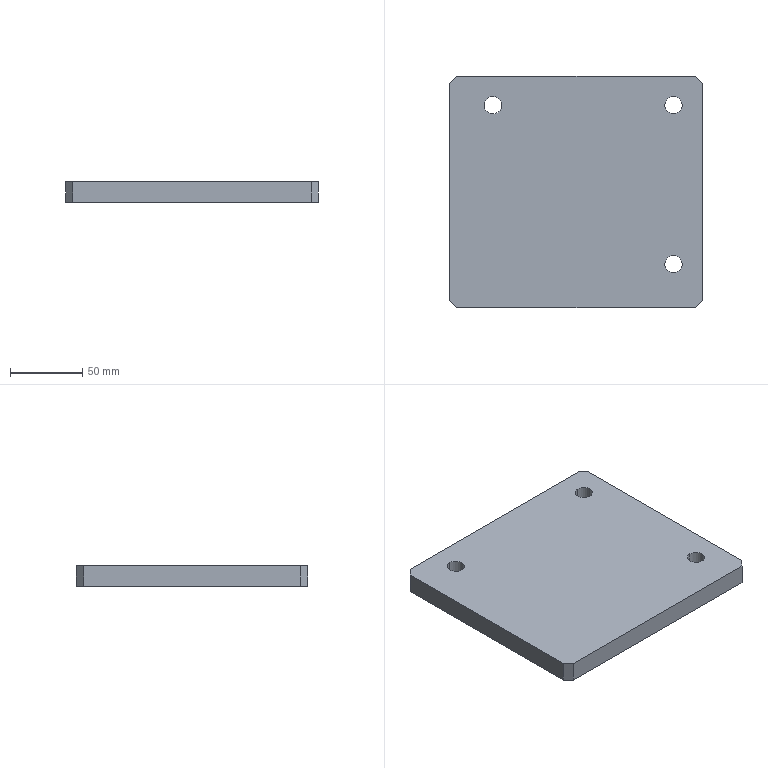Part | STEP file | [08] | 1 solid | 16 faces | box 175 x 160 x 14 mm | volume 386550 mm3 | plane 10 | cylinder 6 | commonest cylinder face diameters 12 x6
STEP:
#1=CARTESIAN_POINT('',(0.,0.,0.));
#2=DIRECTION('',(0.,0.,1.));
#3=DIRECTION('',(1.,0.,0.));
#4=AXIS2_PLACEMENT_3D('',#1,#2,#3);
#5=CARTESIAN_POINT('',(30.,134.,0.));
#6=VERTEX_POINT('',#5);
#7=CARTESIAN_POINT('',(30.,134.,14.));
#8=VERTEX_POINT('',#7);
#9=CARTESIAN_POINT('',(30.,134.,0.));
#10=DIRECTION('',(0.,0.,1.));
#11=VECTOR('',#10,1.);
#12=LINE('',#9,#11);
#13=CARTESIAN_POINT('',(30.,140.,0.));
#14=DIRECTION('',(0.,0.,1.));
#15=DIRECTION('',(0.,-1.,0.));
#16=AXIS2_PLACEMENT_3D('',#13,#14,#15);
#17=CYLINDRICAL_SURFACE('',#16,6.);
#18=CARTESIAN_POINT('',(6.283,0.));
#19=DIRECTION('',(0.,1.));
#20=VECTOR('',#19,1.);
#21=LINE('',#18,#20);
#22=(GEOMETRIC_REPRESENTATION_CONTEXT(2)PARAMETRIC_REPRESENTATION_CONTEXT()REPRESENTATION_CONTEXT('',''));
#23=DEFINITIONAL_REPRESENTATION('',(#21),#22);
#24=PCURVE('',#17,#23);
#25=CARTESIAN_POINT('',(30.,140.,0.));
#26=DIRECTION('',(0.,0.,1.));
#27=DIRECTION('',(0.,-1.,0.));
#28=AXIS2_PLACEMENT_3D('',#25,#26,#27);
#29=CYLINDRICAL_SURFACE('',#28,6.);
#30=CARTESIAN_POINT('',(0.,0.));
#31=DIRECTION('',(0.,1.));
#32=VECTOR('',#31,1.);
#33=LINE('',#30,#32);
#34=(GEOMETRIC_REPRESENTATION_CONTEXT(2)PARAMETRIC_REPRESENTATION_CONTEXT()REPRESENTATION_CONTEXT('',''));
#35=DEFINITIONAL_REPRESENTATION('',(#33),#34);
#36=PCURVE('',#29,#35);
#37=SURFACE_CURVE('',#12,(#24,#36),.PCURVE_S1.);
#38=EDGE_CURVE('',#6,#8,#37,.T.);
#39=ORIENTED_EDGE('',*,*,#38,.T.);
#40=CARTESIAN_POINT('',(30.,146.,14.));
#41=VERTEX_POINT('',#40);
#42=CARTESIAN_POINT('',(30.,140.,14.));
#43=DIRECTION('',(0.,0.,-1.));
#44=DIRECTION('',(0.,1.,0.));
#45=AXIS2_PLACEMENT_3D('',#42,#43,#44);
#46=CIRCLE('',#45,6.);
#47=CARTESIAN_POINT('',(9.425,14.));
#48=DIRECTION('',(-1.,0.));
#49=VECTOR('',#48,1.);
#50=LINE('',#47,#49);
#51=(GEOMETRIC_REPRESENTATION_CONTEXT(2)PARAMETRIC_REPRESENTATION_CONTEXT()REPRESENTATION_CONTEXT('',''));
#52=DEFINITIONAL_REPRESENTATION('',(#50),#51);
#53=PCURVE('',#17,#52);
#54=CARTESIAN_POINT('',(87.5,80.,14.));
#55=DIRECTION('',(0.,0.,1.));
#56=DIRECTION('',(0.,-1.,0.));
#57=AXIS2_PLACEMENT_3D('',#54,#55,#56);
#58=PLANE('',#57);
#59=CARTESIAN_POINT('',(-66.,-57.5));
#60=CARTESIAN_POINT('',(-66.,-47.108));
#61=CARTESIAN_POINT('',(-57.,-52.304));
#62=CARTESIAN_POINT('',(-48.,-57.5));
#63=CARTESIAN_POINT('',(-57.,-62.696));
#64=CARTESIAN_POINT('',(-66.,-67.892));
#65=CARTESIAN_POINT('',(-66.,-57.5));
#66=(BOUNDED_CURVE()B_SPLINE_CURVE(2,(#59,#60,#61,#62,#63,#64,#65),.UNSPECIFIED.,.T.,.F.)B_SPLINE_CURVE_WITH_KNOTS((1,2,2,2,2,1),(-2.094,0.,2.094,4.189,6.283,8.378),.UNSPECIFIED.)CURVE()GEOMETRIC_REPRESENTATION_ITEM()RATIONAL_B_SPLINE_CURVE((1.,0.5,1.,0.5,1.,0.5,1.))REPRESENTATION_ITEM(''));
#67=(GEOMETRIC_REPRESENTATION_CONTEXT(2)PARAMETRIC_REPRESENTATION_CONTEXT()REPRESENTATION_CONTEXT('',''));
#68=DEFINITIONAL_REPRESENTATION('',(#66),#67);
#69=PCURVE('',#58,#68);
#70=SURFACE_CURVE('',#46,(#53,#69),.PCURVE_S1.);
#71=EDGE_CURVE('',#8,#41,#70,.T.);
#72=ORIENTED_EDGE('',*,*,#71,.T.);
#73=CARTESIAN_POINT('',(30.,146.,0.));
#74=VERTEX_POINT('',#73);
#75=CARTESIAN_POINT('',(30.,146.,0.));
#76=DIRECTION('',(0.,0.,1.));
#77=VECTOR('',#76,1.);
#78=LINE('',#75,#77);
#79=CARTESIAN_POINT('',(3.142,0.));
#80=DIRECTION('',(0.,1.));
#81=VECTOR('',#80,1.);
#82=LINE('',#79,#81);
#83=(GEOMETRIC_REPRESENTATION_CONTEXT(2)PARAMETRIC_REPRESENTATION_CONTEXT()REPRESENTATION_CONTEXT('',''));
#84=DEFINITIONAL_REPRESENTATION('',(#82),#83);
#85=PCURVE('',#17,#84);
#86=CARTESIAN_POINT('',(3.142,0.));
#87=DIRECTION('',(0.,1.));
#88=VECTOR('',#87,1.);
#89=LINE('',#86,#88);
#90=(GEOMETRIC_REPRESENTATION_CONTEXT(2)PARAMETRIC_REPRESENTATION_CONTEXT()REPRESENTATION_CONTEXT('',''));
#91=DEFINITIONAL_REPRESENTATION('',(#89),#90);
#92=PCURVE('',#29,#91);
#93=SURFACE_CURVE('',#78,(#85,#92),.PCURVE_S1.);
#94=EDGE_CURVE('',#74,#41,#93,.T.);
#95=ORIENTED_EDGE('',*,*,#94,.F.);
#96=CARTESIAN_POINT('',(30.,140.,0.));
#97=DIRECTION('',(0.,0.,1.));
#98=DIRECTION('',(0.,-1.,0.));
#99=AXIS2_PLACEMENT_3D('',#96,#97,#98);
#100=CIRCLE('',#99,6.);
#101=CARTESIAN_POINT('',(0.,0.));
#102=DIRECTION('',(1.,0.));
#103=VECTOR('',#102,1.);
#104=LINE('',#101,#103);
#105=(GEOMETRIC_REPRESENTATION_CONTEXT(2)PARAMETRIC_REPRESENTATION_CONTEXT()REPRESENTATION_CONTEXT('',''));
#106=DEFINITIONAL_REPRESENTATION('',(#104),#105);
#107=PCURVE('',#17,#106);
#108=CARTESIAN_POINT('',(87.5,80.,0.));
#109=DIRECTION('',(0.,0.,-1.));
#110=DIRECTION('',(0.,1.,0.));
#111=AXIS2_PLACEMENT_3D('',#108,#109,#110);
#112=PLANE('',#111);
#113=CARTESIAN_POINT('',(54.,-57.5));
#114=CARTESIAN_POINT('',(54.,-47.108));
#115=CARTESIAN_POINT('',(63.,-52.304));
#116=CARTESIAN_POINT('',(72.,-57.5));
#117=CARTESIAN_POINT('',(63.,-62.696));
#118=CARTESIAN_POINT('',(54.,-67.892));
#119=CARTESIAN_POINT('',(54.,-57.5));
#120=(BOUNDED_CURVE()B_SPLINE_CURVE(2,(#113,#114,#115,#116,#117,#118,#119),.UNSPECIFIED.,.T.,.F.)B_SPLINE_CURVE_WITH_KNOTS((1,2,2,2,2,1),(-2.094,0.,2.094,4.189,6.283,8.378),.UNSPECIFIED.)CURVE()GEOMETRIC_REPRESENTATION_ITEM()RATIONAL_B_SPLINE_CURVE((1.,0.5,1.,0.5,1.,0.5,1.))REPRESENTATION_ITEM(''));
#121=(GEOMETRIC_REPRESENTATION_CONTEXT(2)PARAMETRIC_REPRESENTATION_CONTEXT()REPRESENTATION_CONTEXT('',''));
#122=DEFINITIONAL_REPRESENTATION('',(#120),#121);
#123=PCURVE('',#112,#122);
#124=SURFACE_CURVE('',#100,(#107,#123),.PCURVE_S1.);
#125=EDGE_CURVE('',#74,#6,#124,.T.);
#126=ORIENTED_EDGE('',*,*,#125,.T.);
#127=EDGE_LOOP('',(#39,#72,#95,#126));
#128=FACE_BOUND('',#127,.F.);
#129=ADVANCED_FACE('',(#128),#17,.F.);
#130=CARTESIAN_POINT('',(155.,24.,0.));
#131=VERTEX_POINT('',#130);
#132=CARTESIAN_POINT('',(155.,24.,14.));
#133=VERTEX_POINT('',#132);
#134=CARTESIAN_POINT('',(155.,24.,0.));
#135=DIRECTION('',(0.,0.,1.));
#136=VECTOR('',#135,1.);
#137=LINE('',#134,#136);
#138=CARTESIAN_POINT('',(155.,30.,0.));
#139=DIRECTION('',(0.,0.,1.));
#140=DIRECTION('',(0.,-1.,0.));
#141=AXIS2_PLACEMENT_3D('',#138,#139,#140);
#142=CYLINDRICAL_SURFACE('',#141,6.);
#143=CARTESIAN_POINT('',(6.283,0.));
#144=DIRECTION('',(0.,1.));
#145=VECTOR('',#144,1.);
#146=LINE('',#143,#145);
#147=(GEOMETRIC_REPRESENTATION_CONTEXT(2)PARAMETRIC_REPRESENTATION_CONTEXT()REPRESENTATION_CONTEXT('',''));
#148=DEFINITIONAL_REPRESENTATION('',(#146),#147);
#149=PCURVE('',#142,#148);
#150=CARTESIAN_POINT('',(155.,30.,0.));
#151=DIRECTION('',(0.,0.,1.));
#152=DIRECTION('',(0.,-1.,0.));
#153=AXIS2_PLACEMENT_3D('',#150,#151,#152);
#154=CYLINDRICAL_SURFACE('',#153,6.);
#155=CARTESIAN_POINT('',(0.,0.));
#156=DIRECTION('',(0.,1.));
#157=VECTOR('',#156,1.);
#158=LINE('',#155,#157);
#159=(GEOMETRIC_REPRESENTATION_CONTEXT(2)PARAMETRIC_REPRESENTATION_CONTEXT()REPRESENTATION_CONTEXT('',''));
#160=DEFINITIONAL_REPRESENTATION('',(#158),#159);
#161=PCURVE('',#154,#160);
#162=SURFACE_CURVE('',#137,(#149,#161),.PCURVE_S1.);
#163=EDGE_CURVE('',#131,#133,#162,.T.);
#164=ORIENTED_EDGE('',*,*,#163,.T.);
#165=CARTESIAN_POINT('',(155.,36.,14.));
#166=VERTEX_POINT('',#165);
#167=CARTESIAN_POINT('',(155.,30.,14.));
#168=DIRECTION('',(0.,0.,-1.));
#169=DIRECTION('',(0.,1.,0.));
#170=AXIS2_PLACEMENT_3D('',#167,#168,#169);
#171=CIRCLE('',#170,6.);
#172=CARTESIAN_POINT('',(9.425,14.));
#173=DIRECTION('',(-1.,0.));
#174=VECTOR('',#173,1.);
#175=LINE('',#172,#174);
#176=(GEOMETRIC_REPRESENTATION_CONTEXT(2)PARAMETRIC_REPRESENTATION_CONTEXT()REPRESENTATION_CONTEXT('',''));
#177=DEFINITIONAL_REPRESENTATION('',(#175),#176);
#178=PCURVE('',#142,#177);
#179=CARTESIAN_POINT('',(44.,67.5));
#180=CARTESIAN_POINT('',(44.,77.892));
#181=CARTESIAN_POINT('',(53.,72.696));
#182=CARTESIAN_POINT('',(62.,67.5));
#183=CARTESIAN_POINT('',(53.,62.304));
#184=CARTESIAN_POINT('',(44.,57.108));
#185=CARTESIAN_POINT('',(44.,67.5));
#186=(BOUNDED_CURVE()B_SPLINE_CURVE(2,(#179,#180,#181,#182,#183,#184,#185),.UNSPECIFIED.,.T.,.F.)B_SPLINE_CURVE_WITH_KNOTS((1,2,2,2,2,1),(-2.094,0.,2.094,4.189,6.283,8.378),.UNSPECIFIED.)CURVE()GEOMETRIC_REPRESENTATION_ITEM()RATIONAL_B_SPLINE_CURVE((1.,0.5,1.,0.5,1.,0.5,1.))REPRESENTATION_ITEM(''));
#187=(GEOMETRIC_REPRESENTATION_CONTEXT(2)PARAMETRIC_REPRESENTATION_CONTEXT()REPRESENTATION_CONTEXT('',''));
#188=DEFINITIONAL_REPRESENTATION('',(#186),#187);
#189=PCURVE('',#58,#188);
#190=SURFACE_CURVE('',#171,(#178,#189),.PCURVE_S1.);
#191=EDGE_CURVE('',#133,#166,#190,.T.);
#192=ORIENTED_EDGE('',*,*,#191,.T.);
#193=CARTESIAN_POINT('',(155.,36.,0.));
#194=VERTEX_POINT('',#193);
#195=CARTESIAN_POINT('',(155.,36.,0.));
#196=DIRECTION('',(0.,0.,1.));
#197=VECTOR('',#196,1.);
#198=LINE('',#195,#197);
#199=CARTESIAN_POINT('',(3.142,0.));
#200=DIRECTION('',(0.,1.));
#201=VECTOR('',#200,1.);
#202=LINE('',#199,#201);
#203=(GEOMETRIC_REPRESENTATION_CONTEXT(2)PARAMETRIC_REPRESENTATION_CONTEXT()REPRESENTATION_CONTEXT('',''));
#204=DEFINITIONAL_REPRESENTATION('',(#202),#203);
#205=PCURVE('',#142,#204);
#206=CARTESIAN_POINT('',(3.142,0.));
#207=DIRECTION('',(0.,1.));
#208=VECTOR('',#207,1.);
#209=LINE('',#206,#208);
#210=(GEOMETRIC_REPRESENTATION_CONTEXT(2)PARAMETRIC_REPRESENTATION_CONTEXT()REPRESENTATION_CONTEXT('',''));
#211=DEFINITIONAL_REPRESENTATION('',(#209),#210);
#212=PCURVE('',#154,#211);
#213=SURFACE_CURVE('',#198,(#205,#212),.PCURVE_S1.);
#214=EDGE_CURVE('',#194,#166,#213,.T.);
#215=ORIENTED_EDGE('',*,*,#214,.F.);
#216=CARTESIAN_POINT('',(155.,30.,0.));
#217=DIRECTION('',(0.,0.,1.));
#218=DIRECTION('',(0.,-1.,0.));
#219=AXIS2_PLACEMENT_3D('',#216,#217,#218);
#220=CIRCLE('',#219,6.);
#221=CARTESIAN_POINT('',(0.,0.));
#222=DIRECTION('',(1.,0.));
#223=VECTOR('',#222,1.);
#224=LINE('',#221,#223);
#225=(GEOMETRIC_REPRESENTATION_CONTEXT(2)PARAMETRIC_REPRESENTATION_CONTEXT()REPRESENTATION_CONTEXT('',''));
#226=DEFINITIONAL_REPRESENTATION('',(#224),#225);
#227=PCURVE('',#142,#226);
#228=CARTESIAN_POINT('',(-56.,67.5));
#229=CARTESIAN_POINT('',(-56.,77.892));
#230=CARTESIAN_POINT('',(-47.,72.696));
#231=CARTESIAN_POINT('',(-38.,67.5));
#232=CARTESIAN_POINT('',(-47.,62.304));
#233=CARTESIAN_POINT('',(-56.,57.108));
#234=CARTESIAN_POINT('',(-56.,67.5));
#235=(BOUNDED_CURVE()B_SPLINE_CURVE(2,(#228,#229,#230,#231,#232,#233,#234),.UNSPECIFIED.,.T.,.F.)B_SPLINE_CURVE_WITH_KNOTS((1,2,2,2,2,1),(-2.094,0.,2.094,4.189,6.283,8.378),.UNSPECIFIED.)CURVE()GEOMETRIC_REPRESENTATION_ITEM()RATIONAL_B_SPLINE_CURVE((1.,0.5,1.,0.5,1.,0.5,1.))REPRESENTATION_ITEM(''));
#236=(GEOMETRIC_REPRESENTATION_CONTEXT(2)PARAMETRIC_REPRESENTATION_CONTEXT()REPRESENTATION_CONTEXT('',''));
#237=DEFINITIONAL_REPRESENTATION('',(#235),#236);
#238=PCURVE('',#112,#237);
#239=SURFACE_CURVE('',#220,(#227,#238),.PCURVE_S1.);
#240=EDGE_CURVE('',#194,#131,#239,.T.);
#241=ORIENTED_EDGE('',*,*,#240,.T.);
#242=EDGE_LOOP('',(#164,#192,#215,#241));
#243=FACE_BOUND('',#242,.F.);
#244=ADVANCED_FACE('',(#243),#142,.F.);
#245=CARTESIAN_POINT('',(155.,134.,0.));
#246=VERTEX_POINT('',#245);
#247=CARTESIAN_POINT('',(155.,134.,14.));
#248=VERTEX_POINT('',#247);
#249=CARTESIAN_POINT('',(155.,134.,0.));
#250=DIRECTION('',(0.,0.,1.));
#251=VECTOR('',#250,1.);
#252=LINE('',#249,#251);
#253=CARTESIAN_POINT('',(155.,140.,0.));
#254=DIRECTION('',(0.,0.,1.));
#255=DIRECTION('',(0.,-1.,0.));
#256=AXIS2_PLACEMENT_3D('',#253,#254,#255);
#257=CYLINDRICAL_SURFACE('',#256,6.);
#258=CARTESIAN_POINT('',(6.283,0.));
#259=DIRECTION('',(0.,1.));
#260=VECTOR('',#259,1.);
#261=LINE('',#258,#260);
#262=(GEOMETRIC_REPRESENTATION_CONTEXT(2)PARAMETRIC_REPRESENTATION_CONTEXT()REPRESENTATION_CONTEXT('',''));
#263=DEFINITIONAL_REPRESENTATION('',(#261),#262);
#264=PCURVE('',#257,#263);
#265=CARTESIAN_POINT('',(155.,140.,0.));
#266=DIRECTION('',(0.,0.,1.));
#267=DIRECTION('',(0.,-1.,0.));
#268=AXIS2_PLACEMENT_3D('',#265,#266,#267);
#269=CYLINDRICAL_SURFACE('',#268,6.);
#270=CARTESIAN_POINT('',(0.,0.));
#271=DIRECTION('',(0.,1.));
#272=VECTOR('',#271,1.);
#273=LINE('',#270,#272);
#274=(GEOMETRIC_REPRESENTATION_CONTEXT(2)PARAMETRIC_REPRESENTATION_CONTEXT()REPRESENTATION_CONTEXT('',''));
#275=DEFINITIONAL_REPRESENTATION('',(#273),#274);
#276=PCURVE('',#269,#275);
#277=SURFACE_CURVE('',#252,(#264,#276),.PCURVE_S1.);
#278=EDGE_CURVE('',#246,#248,#277,.T.);
#279=ORIENTED_EDGE('',*,*,#278,.T.);
#280=CARTESIAN_POINT('',(155.,146.,14.));
#281=VERTEX_POINT('',#280);
#282=CARTESIAN_POINT('',(155.,140.,14.));
#283=DIRECTION('',(0.,0.,-1.));
#284=DIRECTION('',(0.,1.,0.));
#285=AXIS2_PLACEMENT_3D('',#282,#283,#284);
#286=CIRCLE('',#285,6.);
#287=CARTESIAN_POINT('',(9.425,14.));
#288=DIRECTION('',(-1.,0.));
#289=VECTOR('',#288,1.);
#290=LINE('',#287,#289);
#291=(GEOMETRIC_REPRESENTATION_CONTEXT(2)PARAMETRIC_REPRESENTATION_CONTEXT()REPRESENTATION_CONTEXT('',''));
#292=DEFINITIONAL_REPRESENTATION('',(#290),#291);
#293=PCURVE('',#257,#292);
#294=CARTESIAN_POINT('',(-66.,67.5));
#295=CARTESIAN_POINT('',(-66.,77.892));
#296=CARTESIAN_POINT('',(-57.,72.696));
#297=CARTESIAN_POINT('',(-48.,67.5));
#298=CARTESIAN_POINT('',(-57.,62.304));
#299=CARTESIAN_POINT('',(-66.,57.108));
#300=CARTESIAN_POINT('',(-66.,67.5));
#301=(BOUNDED_CURVE()B_SPLINE_CURVE(2,(#294,#295,#296,#297,#298,#299,#300),.UNSPECIFIED.,.T.,.F.)B_SPLINE_CURVE_WITH_KNOTS((1,2,2,2,2,1),(-2.094,0.,2.094,4.189,6.283,8.378),.UNSPECIFIED.)CURVE()GEOMETRIC_REPRESENTATION_ITEM()RATIONAL_B_SPLINE_CURVE((1.,0.5,1.,0.5,1.,0.5,1.))REPRESENTATION_ITEM(''));
#302=(GEOMETRIC_REPRESENTATION_CONTEXT(2)PARAMETRIC_REPRESENTATION_CONTEXT()REPRESENTATION_CONTEXT('',''));
#303=DEFINITIONAL_REPRESENTATION('',(#301),#302);
#304=PCURVE('',#58,#303);
#305=SURFACE_CURVE('',#286,(#293,#304),.PCURVE_S1.);
#306=EDGE_CURVE('',#248,#281,#305,.T.);
#307=ORIENTED_EDGE('',*,*,#306,.T.);
#308=CARTESIAN_POINT('',(155.,146.,0.));
#309=VERTEX_POINT('',#308);
#310=CARTESIAN_POINT('',(155.,146.,0.));
#311=DIRECTION('',(0.,0.,1.));
#312=VECTOR('',#311,1.);
#313=LINE('',#310,#312);
#314=CARTESIAN_POINT('',(3.142,0.));
#315=DIRECTION('',(0.,1.));
#316=VECTOR('',#315,1.);
#317=LINE('',#314,#316);
#318=(GEOMETRIC_REPRESENTATION_CONTEXT(2)PARAMETRIC_REPRESENTATION_CONTEXT()REPRESENTATION_CONTEXT('',''));
#319=DEFINITIONAL_REPRESENTATION('',(#317),#318);
#320=PCURVE('',#257,#319);
#321=CARTESIAN_POINT('',(3.142,0.));
#322=DIRECTION('',(0.,1.));
#323=VECTOR('',#322,1.);
#324=LINE('',#321,#323);
#325=(GEOMETRIC_REPRESENTATION_CONTEXT(2)PARAMETRIC_REPRESENTATION_CONTEXT()REPRESENTATION_CONTEXT('',''));
#326=DEFINITIONAL_REPRESENTATION('',(#324),#325);
#327=PCURVE('',#269,#326);
#328=SURFACE_CURVE('',#313,(#320,#327),.PCURVE_S1.);
#329=EDGE_CURVE('',#309,#281,#328,.T.);
#330=ORIENTED_EDGE('',*,*,#329,.F.);
#331=CARTESIAN_POINT('',(155.,140.,0.));
#332=DIRECTION('',(0.,0.,1.));
#333=DIRECTION('',(0.,-1.,0.));
#334=AXIS2_PLACEMENT_3D('',#331,#332,#333);
#335=CIRCLE('',#334,6.);
#336=CARTESIAN_POINT('',(0.,0.));
#337=DIRECTION('',(1.,0.));
#338=VECTOR('',#337,1.);
#339=LINE('',#336,#338);
#340=(GEOMETRIC_REPRESENTATION_CONTEXT(2)PARAMETRIC_REPRESENTATION_CONTEXT()REPRESENTATION_CONTEXT('',''));
#341=DEFINITIONAL_REPRESENTATION('',(#339),#340);
#342=PCURVE('',#257,#341);
#343=CARTESIAN_POINT('',(54.,67.5));
#344=CARTESIAN_POINT('',(54.,77.892));
#345=CARTESIAN_POINT('',(63.,72.696));
#346=CARTESIAN_POINT('',(72.,67.5));
#347=CARTESIAN_POINT('',(63.,62.304));
#348=CARTESIAN_POINT('',(54.,57.108));
#349=CARTESIAN_POINT('',(54.,67.5));
#350=(BOUNDED_CURVE()B_SPLINE_CURVE(2,(#343,#344,#345,#346,#347,#348,#349),.UNSPECIFIED.,.T.,.F.)B_SPLINE_CURVE_WITH_KNOTS((1,2,2,2,2,1),(-2.094,0.,2.094,4.189,6.283,8.378),.UNSPECIFIED.)CURVE()GEOMETRIC_REPRESENTATION_ITEM()RATIONAL_B_SPLINE_CURVE((1.,0.5,1.,0.5,1.,0.5,1.))REPRESENTATION_ITEM(''));
#351=(GEOMETRIC_REPRESENTATION_CONTEXT(2)PARAMETRIC_REPRESENTATION_CONTEXT()REPRESENTATION_CONTEXT('',''));
#352=DEFINITIONAL_REPRESENTATION('',(#350),#351);
#353=PCURVE('',#112,#352);
#354=SURFACE_CURVE('',#335,(#342,#353),.PCURVE_S1.);
#355=EDGE_CURVE('',#309,#246,#354,.T.);
#356=ORIENTED_EDGE('',*,*,#355,.T.);
#357=EDGE_LOOP('',(#279,#307,#330,#356));
#358=FACE_BOUND('',#357,.F.);
#359=ADVANCED_FACE('',(#358),#257,.F.);
#360=ORIENTED_EDGE('',*,*,#71,.T.);
#361=CARTESIAN_POINT('',(30.,140.,14.));
#362=DIRECTION('',(0.,0.,-1.));
#363=DIRECTION('',(0.,1.,0.));
#364=AXIS2_PLACEMENT_3D('',#361,#362,#363);
#365=CIRCLE('',#364,6.);
#366=CARTESIAN_POINT('',(-66.,-57.5));
#367=CARTESIAN_POINT('',(-66.,-47.108));
#368=CARTESIAN_POINT('',(-57.,-52.304));
#369=CARTESIAN_POINT('',(-48.,-57.5));
#370=CARTESIAN_POINT('',(-57.,-62.696));
#371=CARTESIAN_POINT('',(-66.,-67.892));
#372=CARTESIAN_POINT('',(-66.,-57.5));
#373=(BOUNDED_CURVE()B_SPLINE_CURVE(2,(#366,#367,#368,#369,#370,#371,#372),.UNSPECIFIED.,.T.,.F.)B_SPLINE_CURVE_WITH_KNOTS((1,2,2,2,2,1),(-2.094,0.,2.094,4.189,6.283,8.378),.UNSPECIFIED.)CURVE()GEOMETRIC_REPRESENTATION_ITEM()RATIONAL_B_SPLINE_CURVE((1.,0.5,1.,0.5,1.,0.5,1.))REPRESENTATION_ITEM(''));
#374=(GEOMETRIC_REPRESENTATION_CONTEXT(2)PARAMETRIC_REPRESENTATION_CONTEXT()REPRESENTATION_CONTEXT('',''));
#375=DEFINITIONAL_REPRESENTATION('',(#373),#374);
#376=PCURVE('',#58,#375);
#377=CARTESIAN_POINT('',(3.142,14.));
#378=DIRECTION('',(-1.,0.));
#379=VECTOR('',#378,1.);
#380=LINE('',#377,#379);
#381=(GEOMETRIC_REPRESENTATION_CONTEXT(2)PARAMETRIC_REPRESENTATION_CONTEXT()REPRESENTATION_CONTEXT('',''));
#382=DEFINITIONAL_REPRESENTATION('',(#380),#381);
#383=PCURVE('',#29,#382);
#384=SURFACE_CURVE('',#365,(#376,#383),.PCURVE_S1.);
#385=EDGE_CURVE('',#41,#8,#384,.T.);
#386=ORIENTED_EDGE('',*,*,#385,.T.);
#387=EDGE_LOOP('',(#360,#386));
#388=FACE_BOUND('',#387,.T.);
#389=ORIENTED_EDGE('',*,*,#191,.T.);
#390=CARTESIAN_POINT('',(155.,30.,14.));
#391=DIRECTION('',(0.,0.,-1.));
#392=DIRECTION('',(0.,1.,0.));
#393=AXIS2_PLACEMENT_3D('',#390,#391,#392);
#394=CIRCLE('',#393,6.);
#395=CARTESIAN_POINT('',(44.,67.5));
#396=CARTESIAN_POINT('',(44.,77.892));
#397=CARTESIAN_POINT('',(53.,72.696));
#398=CARTESIAN_POINT('',(62.,67.5));
#399=CARTESIAN_POINT('',(53.,62.304));
#400=CARTESIAN_POINT('',(44.,57.108));
#401=CARTESIAN_POINT('',(44.,67.5));
#402=(BOUNDED_CURVE()B_SPLINE_CURVE(2,(#395,#396,#397,#398,#399,#400,#401),.UNSPECIFIED.,.T.,.F.)B_SPLINE_CURVE_WITH_KNOTS((1,2,2,2,2,1),(-2.094,0.,2.094,4.189,6.283,8.378),.UNSPECIFIED.)CURVE()GEOMETRIC_REPRESENTATION_ITEM()RATIONAL_B_SPLINE_CURVE((1.,0.5,1.,0.5,1.,0.5,1.))REPRESENTATION_ITEM(''));
#403=(GEOMETRIC_REPRESENTATION_CONTEXT(2)PARAMETRIC_REPRESENTATION_CONTEXT()REPRESENTATION_CONTEXT('',''));
#404=DEFINITIONAL_REPRESENTATION('',(#402),#403);
#405=PCURVE('',#58,#404);
#406=CARTESIAN_POINT('',(3.142,14.));
#407=DIRECTION('',(-1.,0.));
#408=VECTOR('',#407,1.);
#409=LINE('',#406,#408);
#410=(GEOMETRIC_REPRESENTATION_CONTEXT(2)PARAMETRIC_REPRESENTATION_CONTEXT()REPRESENTATION_CONTEXT('',''));
#411=DEFINITIONAL_REPRESENTATION('',(#409),#410);
#412=PCURVE('',#154,#411);
#413=SURFACE_CURVE('',#394,(#405,#412),.PCURVE_S1.);
#414=EDGE_CURVE('',#166,#133,#413,.T.);
#415=ORIENTED_EDGE('',*,*,#414,.T.);
#416=EDGE_LOOP('',(#389,#415));
#417=FACE_BOUND('',#416,.T.);
#418=ORIENTED_EDGE('',*,*,#306,.T.);
#419=CARTESIAN_POINT('',(155.,140.,14.));
#420=DIRECTION('',(0.,0.,-1.));
#421=DIRECTION('',(0.,1.,0.));
#422=AXIS2_PLACEMENT_3D('',#419,#420,#421);
#423=CIRCLE('',#422,6.);
#424=CARTESIAN_POINT('',(-66.,67.5));
#425=CARTESIAN_POINT('',(-66.,77.892));
#426=CARTESIAN_POINT('',(-57.,72.696));
#427=CARTESIAN_POINT('',(-48.,67.5));
#428=CARTESIAN_POINT('',(-57.,62.304));
#429=CARTESIAN_POINT('',(-66.,57.108));
#430=CARTESIAN_POINT('',(-66.,67.5));
#431=(BOUNDED_CURVE()B_SPLINE_CURVE(2,(#424,#425,#426,#427,#428,#429,#430),.UNSPECIFIED.,.T.,.F.)B_SPLINE_CURVE_WITH_KNOTS((1,2,2,2,2,1),(-2.094,0.,2.094,4.189,6.283,8.378),.UNSPECIFIED.)CURVE()GEOMETRIC_REPRESENTATION_ITEM()RATIONAL_B_SPLINE_CURVE((1.,0.5,1.,0.5,1.,0.5,1.))REPRESENTATION_ITEM(''));
#432=(GEOMETRIC_REPRESENTATION_CONTEXT(2)PARAMETRIC_REPRESENTATION_CONTEXT()REPRESENTATION_CONTEXT('',''));
#433=DEFINITIONAL_REPRESENTATION('',(#431),#432);
#434=PCURVE('',#58,#433);
#435=CARTESIAN_POINT('',(3.142,14.));
#436=DIRECTION('',(-1.,0.));
#437=VECTOR('',#436,1.);
#438=LINE('',#435,#437);
#439=(GEOMETRIC_REPRESENTATION_CONTEXT(2)PARAMETRIC_REPRESENTATION_CONTEXT()REPRESENTATION_CONTEXT('',''));
#440=DEFINITIONAL_REPRESENTATION('',(#438),#439);
#441=PCURVE('',#269,#440);
#442=SURFACE_CURVE('',#423,(#434,#441),.PCURVE_S1.);
#443=EDGE_CURVE('',#281,#248,#442,.T.);
#444=ORIENTED_EDGE('',*,*,#443,.T.);
#445=EDGE_LOOP('',(#418,#444));
#446=FACE_BOUND('',#445,.T.);
#447=CARTESIAN_POINT('',(170.,0.,14.));
#448=VERTEX_POINT('',#447);
#449=CARTESIAN_POINT('',(5.,0.,14.));
#450=VERTEX_POINT('',#449);
#451=CARTESIAN_POINT('',(87.5,0.,14.));
#452=DIRECTION('',(-1.,0.,0.));
#453=VECTOR('',#452,1.);
#454=LINE('',#451,#453);
#455=CARTESIAN_POINT('',(80.,0.));
#456=DIRECTION('',(0.,-1.));
#457=VECTOR('',#456,1.);
#458=LINE('',#455,#457);
#459=(GEOMETRIC_REPRESENTATION_CONTEXT(2)PARAMETRIC_REPRESENTATION_CONTEXT()REPRESENTATION_CONTEXT('',''));
#460=DEFINITIONAL_REPRESENTATION('',(#458),#459);
#461=PCURVE('',#58,#460);
#462=CARTESIAN_POINT('',(87.5,0.,0.));
#463=DIRECTION('',(0.,-1.,0.));
#464=DIRECTION('',(0.,0.,-1.));
#465=AXIS2_PLACEMENT_3D('',#462,#463,#464);
#466=PLANE('',#465);
#467=CARTESIAN_POINT('',(-14.,0.));
#468=DIRECTION('',(0.,-1.));
#469=VECTOR('',#468,1.);
#470=LINE('',#467,#469);
#471=(GEOMETRIC_REPRESENTATION_CONTEXT(2)PARAMETRIC_REPRESENTATION_CONTEXT()REPRESENTATION_CONTEXT('',''));
#472=DEFINITIONAL_REPRESENTATION('',(#470),#471);
#473=PCURVE('',#466,#472);
#474=SURFACE_CURVE('',#454,(#461,#473),.PCURVE_S1.);
#475=EDGE_CURVE('',#448,#450,#474,.T.);
#476=ORIENTED_EDGE('',*,*,#475,.F.);
#477=CARTESIAN_POINT('',(175.,5.,14.));
#478=VERTEX_POINT('',#477);
#479=CARTESIAN_POINT('',(168.75,-1.25,14.));
#480=DIRECTION('',(0.7071,0.7071,0.));
#481=VECTOR('',#480,1.);
#482=LINE('',#479,#481);
#483=CARTESIAN_POINT('',(81.25,81.25));
#484=DIRECTION('',(-0.7071,0.7071));
#485=VECTOR('',#484,1.);
#486=LINE('',#483,#485);
#487=(GEOMETRIC_REPRESENTATION_CONTEXT(2)PARAMETRIC_REPRESENTATION_CONTEXT()REPRESENTATION_CONTEXT('',''));
#488=DEFINITIONAL_REPRESENTATION('',(#486),#487);
#489=PCURVE('',#58,#488);
#490=CARTESIAN_POINT('',(170.,0.,0.));
#491=DIRECTION('',(-0.7071,0.7071,0.));
#492=DIRECTION('',(0.,0.,1.));
#493=AXIS2_PLACEMENT_3D('',#490,#491,#492);
#494=PLANE('',#493);
#495=CARTESIAN_POINT('',(14.,-1.768));
#496=DIRECTION('',(0.,1.));
#497=VECTOR('',#496,1.);
#498=LINE('',#495,#497);
#499=(GEOMETRIC_REPRESENTATION_CONTEXT(2)PARAMETRIC_REPRESENTATION_CONTEXT()REPRESENTATION_CONTEXT('',''));
#500=DEFINITIONAL_REPRESENTATION('',(#498),#499);
#501=PCURVE('',#494,#500);
#502=SURFACE_CURVE('',#482,(#489,#501),.PCURVE_S1.);
#503=EDGE_CURVE('',#448,#478,#502,.T.);
#504=ORIENTED_EDGE('',*,*,#503,.T.);
#505=CARTESIAN_POINT('',(175.,155.,14.));
#506=VERTEX_POINT('',#505);
#507=CARTESIAN_POINT('',(175.,80.,14.));
#508=DIRECTION('',(0.,-1.,0.));
#509=VECTOR('',#508,1.);
#510=LINE('',#507,#509);
#511=CARTESIAN_POINT('',(0.,87.5));
#512=DIRECTION('',(1.,0.));
#513=VECTOR('',#512,1.);
#514=LINE('',#511,#513);
#515=(GEOMETRIC_REPRESENTATION_CONTEXT(2)PARAMETRIC_REPRESENTATION_CONTEXT()REPRESENTATION_CONTEXT('',''));
#516=DEFINITIONAL_REPRESENTATION('',(#514),#515);
#517=PCURVE('',#58,#516);
#518=CARTESIAN_POINT('',(175.,80.,0.));
#519=DIRECTION('',(1.,0.,0.));
#520=DIRECTION('',(0.,0.,1.));
#521=AXIS2_PLACEMENT_3D('',#518,#519,#520);
#522=PLANE('',#521);
#523=CARTESIAN_POINT('',(14.,0.));
#524=DIRECTION('',(0.,1.));
#525=VECTOR('',#524,1.);
#526=LINE('',#523,#525);
#527=(GEOMETRIC_REPRESENTATION_CONTEXT(2)PARAMETRIC_REPRESENTATION_CONTEXT()REPRESENTATION_CONTEXT('',''));
#528=DEFINITIONAL_REPRESENTATION('',(#526),#527);
#529=PCURVE('',#522,#528);
#530=SURFACE_CURVE('',#510,(#517,#529),.PCURVE_S1.);
#531=EDGE_CURVE('',#506,#478,#530,.T.);
#532=ORIENTED_EDGE('',*,*,#531,.F.);
#533=CARTESIAN_POINT('',(170.,160.,14.));
#534=VERTEX_POINT('',#533);
#535=CARTESIAN_POINT('',(168.75,161.25,14.));
#536=DIRECTION('',(-0.7071,0.7071,0.));
#537=VECTOR('',#536,1.);
#538=LINE('',#535,#537);
#539=CARTESIAN_POINT('',(-81.25,81.25));
#540=DIRECTION('',(-0.7071,-0.7071));
#541=VECTOR('',#540,1.);
#542=LINE('',#539,#541);
#543=(GEOMETRIC_REPRESENTATION_CONTEXT(2)PARAMETRIC_REPRESENTATION_CONTEXT()REPRESENTATION_CONTEXT('',''));
#544=DEFINITIONAL_REPRESENTATION('',(#542),#543);
#545=PCURVE('',#58,#544);
#546=CARTESIAN_POINT('',(175.,155.,0.));
#547=DIRECTION('',(-0.7071,-0.7071,0.));
#548=DIRECTION('',(0.,0.,1.));
#549=AXIS2_PLACEMENT_3D('',#546,#547,#548);
#550=PLANE('',#549);
#551=CARTESIAN_POINT('',(14.,8.839));
#552=DIRECTION('',(0.,1.));
#553=VECTOR('',#552,1.);
#554=LINE('',#551,#553);
#555=(GEOMETRIC_REPRESENTATION_CONTEXT(2)PARAMETRIC_REPRESENTATION_CONTEXT()REPRESENTATION_CONTEXT('',''));
#556=DEFINITIONAL_REPRESENTATION('',(#554),#555);
#557=PCURVE('',#550,#556);
#558=SURFACE_CURVE('',#538,(#545,#557),.PCURVE_S1.);
#559=EDGE_CURVE('',#506,#534,#558,.T.);
#560=ORIENTED_EDGE('',*,*,#559,.T.);
#561=CARTESIAN_POINT('',(5.,160.,14.));
#562=VERTEX_POINT('',#561);
#563=CARTESIAN_POINT('',(87.5,160.,14.));
#564=DIRECTION('',(1.,0.,0.));
#565=VECTOR('',#564,1.);
#566=LINE('',#563,#565);
#567=CARTESIAN_POINT('',(-80.,0.));
#568=DIRECTION('',(0.,1.));
#569=VECTOR('',#568,1.);
#570=LINE('',#567,#569);
#571=(GEOMETRIC_REPRESENTATION_CONTEXT(2)PARAMETRIC_REPRESENTATION_CONTEXT()REPRESENTATION_CONTEXT('',''));
#572=DEFINITIONAL_REPRESENTATION('',(#570),#571);
#573=PCURVE('',#58,#572);
#574=CARTESIAN_POINT('',(87.5,160.,0.));
#575=DIRECTION('',(0.,1.,0.));
#576=DIRECTION('',(0.,0.,1.));
#577=AXIS2_PLACEMENT_3D('',#574,#575,#576);
#578=PLANE('',#577);
#579=CARTESIAN_POINT('',(14.,0.));
#580=DIRECTION('',(0.,1.));
#581=VECTOR('',#580,1.);
#582=LINE('',#579,#581);
#583=(GEOMETRIC_REPRESENTATION_CONTEXT(2)PARAMETRIC_REPRESENTATION_CONTEXT()REPRESENTATION_CONTEXT('',''));
#584=DEFINITIONAL_REPRESENTATION('',(#582),#583);
#585=PCURVE('',#578,#584);
#586=SURFACE_CURVE('',#566,(#573,#585),.PCURVE_S1.);
#587=EDGE_CURVE('',#562,#534,#586,.T.);
#588=ORIENTED_EDGE('',*,*,#587,.F.);
#589=CARTESIAN_POINT('',(0.,155.,14.));
#590=VERTEX_POINT('',#589);
#591=CARTESIAN_POINT('',(6.25,161.25,14.));
#592=DIRECTION('',(-0.7071,-0.7071,0.));
#593=VECTOR('',#592,1.);
#594=LINE('',#591,#593);
#595=CARTESIAN_POINT('',(-81.25,-81.25));
#596=DIRECTION('',(0.7071,-0.7071));
#597=VECTOR('',#596,1.);
#598=LINE('',#595,#597);
#599=(GEOMETRIC_REPRESENTATION_CONTEXT(2)PARAMETRIC_REPRESENTATION_CONTEXT()REPRESENTATION_CONTEXT('',''));
#600=DEFINITIONAL_REPRESENTATION('',(#598),#599);
#601=PCURVE('',#58,#600);
#602=CARTESIAN_POINT('',(5.,160.,0.));
#603=DIRECTION('',(0.7071,-0.7071,0.));
#604=DIRECTION('',(0.,0.,1.));
#605=AXIS2_PLACEMENT_3D('',#602,#603,#604);
#606=PLANE('',#605);
#607=CARTESIAN_POINT('',(14.,-1.768));
#608=DIRECTION('',(0.,1.));
#609=VECTOR('',#608,1.);
#610=LINE('',#607,#609);
#611=(GEOMETRIC_REPRESENTATION_CONTEXT(2)PARAMETRIC_REPRESENTATION_CONTEXT()REPRESENTATION_CONTEXT('',''));
#612=DEFINITIONAL_REPRESENTATION('',(#610),#611);
#613=PCURVE('',#606,#612);
#614=SURFACE_CURVE('',#594,(#601,#613),.PCURVE_S1.);
#615=EDGE_CURVE('',#562,#590,#614,.T.);
#616=ORIENTED_EDGE('',*,*,#615,.T.);
#617=CARTESIAN_POINT('',(0.,5.,14.));
#618=VERTEX_POINT('',#617);
#619=CARTESIAN_POINT('',(0.,80.,14.));
#620=DIRECTION('',(0.,1.,0.));
#621=VECTOR('',#620,1.);
#622=LINE('',#619,#621);
#623=CARTESIAN_POINT('',(0.,-87.5));
#624=DIRECTION('',(-1.,0.));
#625=VECTOR('',#624,1.);
#626=LINE('',#623,#625);
#627=(GEOMETRIC_REPRESENTATION_CONTEXT(2)PARAMETRIC_REPRESENTATION_CONTEXT()REPRESENTATION_CONTEXT('',''));
#628=DEFINITIONAL_REPRESENTATION('',(#626),#627);
#629=PCURVE('',#58,#628);
#630=CARTESIAN_POINT('',(0.,80.,0.));
#631=DIRECTION('',(-1.,0.,0.));
#632=DIRECTION('',(0.,0.,-1.));
#633=AXIS2_PLACEMENT_3D('',#630,#631,#632);
#634=PLANE('',#633);
#635=CARTESIAN_POINT('',(-14.,0.));
#636=DIRECTION('',(0.,-1.));
#637=VECTOR('',#636,1.);
#638=LINE('',#635,#637);
#639=(GEOMETRIC_REPRESENTATION_CONTEXT(2)PARAMETRIC_REPRESENTATION_CONTEXT()REPRESENTATION_CONTEXT('',''));
#640=DEFINITIONAL_REPRESENTATION('',(#638),#639);
#641=PCURVE('',#634,#640);
#642=SURFACE_CURVE('',#622,(#629,#641),.PCURVE_S1.);
#643=EDGE_CURVE('',#618,#590,#642,.T.);
#644=ORIENTED_EDGE('',*,*,#643,.F.);
#645=CARTESIAN_POINT('',(6.25,-1.25,14.));
#646=DIRECTION('',(0.7071,-0.7071,0.));
#647=VECTOR('',#646,1.);
#648=LINE('',#645,#647);
#649=CARTESIAN_POINT('',(81.25,-81.25));
#650=DIRECTION('',(0.7071,0.7071));
#651=VECTOR('',#650,1.);
#652=LINE('',#649,#651);
#653=(GEOMETRIC_REPRESENTATION_CONTEXT(2)PARAMETRIC_REPRESENTATION_CONTEXT()REPRESENTATION_CONTEXT('',''));
#654=DEFINITIONAL_REPRESENTATION('',(#652),#653);
#655=PCURVE('',#58,#654);
#656=CARTESIAN_POINT('',(0.,5.,0.));
#657=DIRECTION('',(0.7071,0.7071,0.));
#658=DIRECTION('',(0.,0.,1.));
#659=AXIS2_PLACEMENT_3D('',#656,#657,#658);
#660=PLANE('',#659);
#661=CARTESIAN_POINT('',(14.,8.839));
#662=DIRECTION('',(0.,1.));
#663=VECTOR('',#662,1.);
#664=LINE('',#661,#663);
#665=(GEOMETRIC_REPRESENTATION_CONTEXT(2)PARAMETRIC_REPRESENTATION_CONTEXT()REPRESENTATION_CONTEXT('',''));
#666=DEFINITIONAL_REPRESENTATION('',(#664),#665);
#667=PCURVE('',#660,#666);
#668=SURFACE_CURVE('',#648,(#655,#667),.PCURVE_S1.);
#669=EDGE_CURVE('',#618,#450,#668,.T.);
#670=ORIENTED_EDGE('',*,*,#669,.T.);
#671=EDGE_LOOP('',(#476,#504,#532,#560,#588,#616,#644,#670));
#672=FACE_BOUND('',#671,.T.);
#673=ADVANCED_FACE('',(#388,#417,#446,#672),#58,.T.);
#674=ORIENTED_EDGE('',*,*,#643,.T.);
#675=CARTESIAN_POINT('',(0.,155.,0.));
#676=VERTEX_POINT('',#675);
#677=CARTESIAN_POINT('',(0.,155.,0.));
#678=DIRECTION('',(0.,0.,-1.));
#679=VECTOR('',#678,1.);
#680=LINE('',#677,#679);
#681=CARTESIAN_POINT('',(0.,-75.));
#682=DIRECTION('',(1.,0.));
#683=VECTOR('',#682,1.);
#684=LINE('',#681,#683);
#685=(GEOMETRIC_REPRESENTATION_CONTEXT(2)PARAMETRIC_REPRESENTATION_CONTEXT()REPRESENTATION_CONTEXT('',''));
#686=DEFINITIONAL_REPRESENTATION('',(#684),#685);
#687=PCURVE('',#634,#686);
#688=CARTESIAN_POINT('',(0.,7.071));
#689=DIRECTION('',(-1.,0.));
#690=VECTOR('',#689,1.);
#691=LINE('',#688,#690);
#692=(GEOMETRIC_REPRESENTATION_CONTEXT(2)PARAMETRIC_REPRESENTATION_CONTEXT()REPRESENTATION_CONTEXT('',''));
#693=DEFINITIONAL_REPRESENTATION('',(#691),#692);
#694=PCURVE('',#606,#693);
#695=SURFACE_CURVE('',#680,(#687,#694),.PCURVE_S1.);
#696=EDGE_CURVE('',#590,#676,#695,.T.);
#697=ORIENTED_EDGE('',*,*,#696,.T.);
#698=CARTESIAN_POINT('',(0.,5.,0.));
#699=VERTEX_POINT('',#698);
#700=CARTESIAN_POINT('',(0.,80.,0.));
#701=DIRECTION('',(0.,-1.,0.));
#702=VECTOR('',#701,1.);
#703=LINE('',#700,#702);
#704=CARTESIAN_POINT('',(0.,0.));
#705=DIRECTION('',(0.,1.));
#706=VECTOR('',#705,1.);
#707=LINE('',#704,#706);
#708=(GEOMETRIC_REPRESENTATION_CONTEXT(2)PARAMETRIC_REPRESENTATION_CONTEXT()REPRESENTATION_CONTEXT('',''));
#709=DEFINITIONAL_REPRESENTATION('',(#707),#708);
#710=PCURVE('',#634,#709);
#711=CARTESIAN_POINT('',(0.,-87.5));
#712=DIRECTION('',(-1.,0.));
#713=VECTOR('',#712,1.);
#714=LINE('',#711,#713);
#715=(GEOMETRIC_REPRESENTATION_CONTEXT(2)PARAMETRIC_REPRESENTATION_CONTEXT()REPRESENTATION_CONTEXT('',''));
#716=DEFINITIONAL_REPRESENTATION('',(#714),#715);
#717=PCURVE('',#112,#716);
#718=SURFACE_CURVE('',#703,(#710,#717),.PCURVE_S1.);
#719=EDGE_CURVE('',#676,#699,#718,.T.);
#720=ORIENTED_EDGE('',*,*,#719,.T.);
#721=CARTESIAN_POINT('',(0.,5.,0.));
#722=DIRECTION('',(0.,0.,1.));
#723=VECTOR('',#722,1.);
#724=LINE('',#721,#723);
#725=CARTESIAN_POINT('',(0.,75.));
#726=DIRECTION('',(-1.,0.));
#727=VECTOR('',#726,1.);
#728=LINE('',#725,#727);
#729=(GEOMETRIC_REPRESENTATION_CONTEXT(2)PARAMETRIC_REPRESENTATION_CONTEXT()REPRESENTATION_CONTEXT('',''));
#730=DEFINITIONAL_REPRESENTATION('',(#728),#729);
#731=PCURVE('',#634,#730);
#732=CARTESIAN_POINT('',(0.,0.));
#733=DIRECTION('',(1.,0.));
#734=VECTOR('',#733,1.);
#735=LINE('',#732,#734);
#736=(GEOMETRIC_REPRESENTATION_CONTEXT(2)PARAMETRIC_REPRESENTATION_CONTEXT()REPRESENTATION_CONTEXT('',''));
#737=DEFINITIONAL_REPRESENTATION('',(#735),#736);
#738=PCURVE('',#660,#737);
#739=SURFACE_CURVE('',#724,(#731,#738),.PCURVE_S1.);
#740=EDGE_CURVE('',#699,#618,#739,.T.);
#741=ORIENTED_EDGE('',*,*,#740,.T.);
#742=EDGE_LOOP('',(#674,#697,#720,#741));
#743=FACE_BOUND('',#742,.T.);
#744=ADVANCED_FACE('',(#743),#634,.T.);
#745=ORIENTED_EDGE('',*,*,#587,.T.);
#746=CARTESIAN_POINT('',(170.,160.,0.));
#747=VERTEX_POINT('',#746);
#748=CARTESIAN_POINT('',(170.,160.,0.));
#749=DIRECTION('',(0.,0.,-1.));
#750=VECTOR('',#749,1.);
#751=LINE('',#748,#750);
#752=CARTESIAN_POINT('',(0.,82.5));
#753=DIRECTION('',(-1.,0.));
#754=VECTOR('',#753,1.);
#755=LINE('',#752,#754);
#756=(GEOMETRIC_REPRESENTATION_CONTEXT(2)PARAMETRIC_REPRESENTATION_CONTEXT()REPRESENTATION_CONTEXT('',''));
#757=DEFINITIONAL_REPRESENTATION('',(#755),#756);
#758=PCURVE('',#578,#757);
#759=CARTESIAN_POINT('',(0.,7.071));
#760=DIRECTION('',(-1.,0.));
#761=VECTOR('',#760,1.);
#762=LINE('',#759,#761);
#763=(GEOMETRIC_REPRESENTATION_CONTEXT(2)PARAMETRIC_REPRESENTATION_CONTEXT()REPRESENTATION_CONTEXT('',''));
#764=DEFINITIONAL_REPRESENTATION('',(#762),#763);
#765=PCURVE('',#550,#764);
#766=SURFACE_CURVE('',#751,(#758,#765),.PCURVE_S1.);
#767=EDGE_CURVE('',#534,#747,#766,.T.);
#768=ORIENTED_EDGE('',*,*,#767,.T.);
#769=CARTESIAN_POINT('',(5.,160.,0.));
#770=VERTEX_POINT('',#769);
#771=CARTESIAN_POINT('',(87.5,160.,0.));
#772=DIRECTION('',(-1.,0.,0.));
#773=VECTOR('',#772,1.);
#774=LINE('',#771,#773);
#775=CARTESIAN_POINT('',(0.,0.));
#776=DIRECTION('',(0.,-1.));
#777=VECTOR('',#776,1.);
#778=LINE('',#775,#777);
#779=(GEOMETRIC_REPRESENTATION_CONTEXT(2)PARAMETRIC_REPRESENTATION_CONTEXT()REPRESENTATION_CONTEXT('',''));
#780=DEFINITIONAL_REPRESENTATION('',(#778),#779);
#781=PCURVE('',#578,#780);
#782=CARTESIAN_POINT('',(80.,0.));
#783=DIRECTION('',(0.,-1.));
#784=VECTOR('',#783,1.);
#785=LINE('',#782,#784);
#786=(GEOMETRIC_REPRESENTATION_CONTEXT(2)PARAMETRIC_REPRESENTATION_CONTEXT()REPRESENTATION_CONTEXT('',''));
#787=DEFINITIONAL_REPRESENTATION('',(#785),#786);
#788=PCURVE('',#112,#787);
#789=SURFACE_CURVE('',#774,(#781,#788),.PCURVE_S1.);
#790=EDGE_CURVE('',#747,#770,#789,.T.);
#791=ORIENTED_EDGE('',*,*,#790,.T.);
#792=CARTESIAN_POINT('',(5.,160.,0.));
#793=DIRECTION('',(0.,0.,1.));
#794=VECTOR('',#793,1.);
#795=LINE('',#792,#794);
#796=CARTESIAN_POINT('',(0.,-82.5));
#797=DIRECTION('',(1.,0.));
#798=VECTOR('',#797,1.);
#799=LINE('',#796,#798);
#800=(GEOMETRIC_REPRESENTATION_CONTEXT(2)PARAMETRIC_REPRESENTATION_CONTEXT()REPRESENTATION_CONTEXT('',''));
#801=DEFINITIONAL_REPRESENTATION('',(#799),#800);
#802=PCURVE('',#578,#801);
#803=CARTESIAN_POINT('',(0.,0.));
#804=DIRECTION('',(1.,0.));
#805=VECTOR('',#804,1.);
#806=LINE('',#803,#805);
#807=(GEOMETRIC_REPRESENTATION_CONTEXT(2)PARAMETRIC_REPRESENTATION_CONTEXT()REPRESENTATION_CONTEXT('',''));
#808=DEFINITIONAL_REPRESENTATION('',(#806),#807);
#809=PCURVE('',#606,#808);
#810=SURFACE_CURVE('',#795,(#802,#809),.PCURVE_S1.);
#811=EDGE_CURVE('',#770,#562,#810,.T.);
#812=ORIENTED_EDGE('',*,*,#811,.T.);
#813=EDGE_LOOP('',(#745,#768,#791,#812));
#814=FACE_BOUND('',#813,.T.);
#815=ADVANCED_FACE('',(#814),#578,.T.);
#816=ORIENTED_EDGE('',*,*,#531,.T.);
#817=CARTESIAN_POINT('',(175.,5.,0.));
#818=VERTEX_POINT('',#817);
#819=CARTESIAN_POINT('',(175.,5.,0.));
#820=DIRECTION('',(0.,0.,-1.));
#821=VECTOR('',#820,1.);
#822=LINE('',#819,#821);
#823=CARTESIAN_POINT('',(0.,75.));
#824=DIRECTION('',(-1.,0.));
#825=VECTOR('',#824,1.);
#826=LINE('',#823,#825);
#827=(GEOMETRIC_REPRESENTATION_CONTEXT(2)PARAMETRIC_REPRESENTATION_CONTEXT()REPRESENTATION_CONTEXT('',''));
#828=DEFINITIONAL_REPRESENTATION('',(#826),#827);
#829=PCURVE('',#522,#828);
#830=CARTESIAN_POINT('',(0.,7.071));
#831=DIRECTION('',(-1.,0.));
#832=VECTOR('',#831,1.);
#833=LINE('',#830,#832);
#834=(GEOMETRIC_REPRESENTATION_CONTEXT(2)PARAMETRIC_REPRESENTATION_CONTEXT()REPRESENTATION_CONTEXT('',''));
#835=DEFINITIONAL_REPRESENTATION('',(#833),#834);
#836=PCURVE('',#494,#835);
#837=SURFACE_CURVE('',#822,(#829,#836),.PCURVE_S1.);
#838=EDGE_CURVE('',#478,#818,#837,.T.);
#839=ORIENTED_EDGE('',*,*,#838,.T.);
#840=CARTESIAN_POINT('',(175.,155.,0.));
#841=VERTEX_POINT('',#840);
#842=CARTESIAN_POINT('',(175.,80.,0.));
#843=DIRECTION('',(0.,1.,0.));
#844=VECTOR('',#843,1.);
#845=LINE('',#842,#844);
#846=CARTESIAN_POINT('',(0.,0.));
#847=DIRECTION('',(0.,-1.));
#848=VECTOR('',#847,1.);
#849=LINE('',#846,#848);
#850=(GEOMETRIC_REPRESENTATION_CONTEXT(2)PARAMETRIC_REPRESENTATION_CONTEXT()REPRESENTATION_CONTEXT('',''));
#851=DEFINITIONAL_REPRESENTATION('',(#849),#850);
#852=PCURVE('',#522,#851);
#853=CARTESIAN_POINT('',(0.,87.5));
#854=DIRECTION('',(1.,0.));
#855=VECTOR('',#854,1.);
#856=LINE('',#853,#855);
#857=(GEOMETRIC_REPRESENTATION_CONTEXT(2)PARAMETRIC_REPRESENTATION_CONTEXT()REPRESENTATION_CONTEXT('',''));
#858=DEFINITIONAL_REPRESENTATION('',(#856),#857);
#859=PCURVE('',#112,#858);
#860=SURFACE_CURVE('',#845,(#852,#859),.PCURVE_S1.);
#861=EDGE_CURVE('',#818,#841,#860,.T.);
#862=ORIENTED_EDGE('',*,*,#861,.T.);
#863=CARTESIAN_POINT('',(175.,155.,0.));
#864=DIRECTION('',(0.,0.,1.));
#865=VECTOR('',#864,1.);
#866=LINE('',#863,#865);
#867=CARTESIAN_POINT('',(0.,-75.));
#868=DIRECTION('',(1.,0.));
#869=VECTOR('',#868,1.);
#870=LINE('',#867,#869);
#871=(GEOMETRIC_REPRESENTATION_CONTEXT(2)PARAMETRIC_REPRESENTATION_CONTEXT()REPRESENTATION_CONTEXT('',''));
#872=DEFINITIONAL_REPRESENTATION('',(#870),#871);
#873=PCURVE('',#522,#872);
#874=CARTESIAN_POINT('',(0.,0.));
#875=DIRECTION('',(1.,0.));
#876=VECTOR('',#875,1.);
#877=LINE('',#874,#876);
#878=(GEOMETRIC_REPRESENTATION_CONTEXT(2)PARAMETRIC_REPRESENTATION_CONTEXT()REPRESENTATION_CONTEXT('',''));
#879=DEFINITIONAL_REPRESENTATION('',(#877),#878);
#880=PCURVE('',#550,#879);
#881=SURFACE_CURVE('',#866,(#873,#880),.PCURVE_S1.);
#882=EDGE_CURVE('',#841,#506,#881,.T.);
#883=ORIENTED_EDGE('',*,*,#882,.T.);
#884=EDGE_LOOP('',(#816,#839,#862,#883));
#885=FACE_BOUND('',#884,.T.);
#886=ADVANCED_FACE('',(#885),#522,.T.);
#887=CARTESIAN_POINT('',(30.,140.,0.));
#888=DIRECTION('',(0.,0.,1.));
#889=DIRECTION('',(0.,-1.,0.));
#890=AXIS2_PLACEMENT_3D('',#887,#888,#889);
#891=CIRCLE('',#890,6.);
#892=CARTESIAN_POINT('',(54.,-57.5));
#893=CARTESIAN_POINT('',(54.,-47.108));
#894=CARTESIAN_POINT('',(63.,-52.304));
#895=CARTESIAN_POINT('',(72.,-57.5));
#896=CARTESIAN_POINT('',(63.,-62.696));
#897=CARTESIAN_POINT('',(54.,-67.892));
#898=CARTESIAN_POINT('',(54.,-57.5));
#899=(BOUNDED_CURVE()B_SPLINE_CURVE(2,(#892,#893,#894,#895,#896,#897,#898),.UNSPECIFIED.,.T.,.F.)B_SPLINE_CURVE_WITH_KNOTS((1,2,2,2,2,1),(-2.094,0.,2.094,4.189,6.283,8.378),.UNSPECIFIED.)CURVE()GEOMETRIC_REPRESENTATION_ITEM()RATIONAL_B_SPLINE_CURVE((1.,0.5,1.,0.5,1.,0.5,1.))REPRESENTATION_ITEM(''));
#900=(GEOMETRIC_REPRESENTATION_CONTEXT(2)PARAMETRIC_REPRESENTATION_CONTEXT()REPRESENTATION_CONTEXT('',''));
#901=DEFINITIONAL_REPRESENTATION('',(#899),#900);
#902=PCURVE('',#112,#901);
#903=CARTESIAN_POINT('',(0.,0.));
#904=DIRECTION('',(1.,0.));
#905=VECTOR('',#904,1.);
#906=LINE('',#903,#905);
#907=(GEOMETRIC_REPRESENTATION_CONTEXT(2)PARAMETRIC_REPRESENTATION_CONTEXT()REPRESENTATION_CONTEXT('',''));
#908=DEFINITIONAL_REPRESENTATION('',(#906),#907);
#909=PCURVE('',#29,#908);
#910=SURFACE_CURVE('',#891,(#902,#909),.PCURVE_S1.);
#911=EDGE_CURVE('',#6,#74,#910,.T.);
#912=ORIENTED_EDGE('',*,*,#911,.T.);
#913=ORIENTED_EDGE('',*,*,#125,.T.);
#914=EDGE_LOOP('',(#912,#913));
#915=FACE_BOUND('',#914,.T.);
#916=CARTESIAN_POINT('',(155.,30.,0.));
#917=DIRECTION('',(0.,0.,1.));
#918=DIRECTION('',(0.,-1.,0.));
#919=AXIS2_PLACEMENT_3D('',#916,#917,#918);
#920=CIRCLE('',#919,6.);
#921=CARTESIAN_POINT('',(-56.,67.5));
#922=CARTESIAN_POINT('',(-56.,77.892));
#923=CARTESIAN_POINT('',(-47.,72.696));
#924=CARTESIAN_POINT('',(-38.,67.5));
#925=CARTESIAN_POINT('',(-47.,62.304));
#926=CARTESIAN_POINT('',(-56.,57.108));
#927=CARTESIAN_POINT('',(-56.,67.5));
#928=(BOUNDED_CURVE()B_SPLINE_CURVE(2,(#921,#922,#923,#924,#925,#926,#927),.UNSPECIFIED.,.T.,.F.)B_SPLINE_CURVE_WITH_KNOTS((1,2,2,2,2,1),(-2.094,0.,2.094,4.189,6.283,8.378),.UNSPECIFIED.)CURVE()GEOMETRIC_REPRESENTATION_ITEM()RATIONAL_B_SPLINE_CURVE((1.,0.5,1.,0.5,1.,0.5,1.))REPRESENTATION_ITEM(''));
#929=(GEOMETRIC_REPRESENTATION_CONTEXT(2)PARAMETRIC_REPRESENTATION_CONTEXT()REPRESENTATION_CONTEXT('',''));
#930=DEFINITIONAL_REPRESENTATION('',(#928),#929);
#931=PCURVE('',#112,#930);
#932=CARTESIAN_POINT('',(0.,0.));
#933=DIRECTION('',(1.,0.));
#934=VECTOR('',#933,1.);
#935=LINE('',#932,#934);
#936=(GEOMETRIC_REPRESENTATION_CONTEXT(2)PARAMETRIC_REPRESENTATION_CONTEXT()REPRESENTATION_CONTEXT('',''));
#937=DEFINITIONAL_REPRESENTATION('',(#935),#936);
#938=PCURVE('',#154,#937);
#939=SURFACE_CURVE('',#920,(#931,#938),.PCURVE_S1.);
#940=EDGE_CURVE('',#131,#194,#939,.T.);
#941=ORIENTED_EDGE('',*,*,#940,.T.);
#942=ORIENTED_EDGE('',*,*,#240,.T.);
#943=EDGE_LOOP('',(#941,#942));
#944=FACE_BOUND('',#943,.T.);
#945=CARTESIAN_POINT('',(155.,140.,0.));
#946=DIRECTION('',(0.,0.,1.));
#947=DIRECTION('',(0.,-1.,0.));
#948=AXIS2_PLACEMENT_3D('',#945,#946,#947);
#949=CIRCLE('',#948,6.);
#950=CARTESIAN_POINT('',(54.,67.5));
#951=CARTESIAN_POINT('',(54.,77.892));
#952=CARTESIAN_POINT('',(63.,72.696));
#953=CARTESIAN_POINT('',(72.,67.5));
#954=CARTESIAN_POINT('',(63.,62.304));
#955=CARTESIAN_POINT('',(54.,57.108));
#956=CARTESIAN_POINT('',(54.,67.5));
#957=(BOUNDED_CURVE()B_SPLINE_CURVE(2,(#950,#951,#952,#953,#954,#955,#956),.UNSPECIFIED.,.T.,.F.)B_SPLINE_CURVE_WITH_KNOTS((1,2,2,2,2,1),(-2.094,0.,2.094,4.189,6.283,8.378),.UNSPECIFIED.)CURVE()GEOMETRIC_REPRESENTATION_ITEM()RATIONAL_B_SPLINE_CURVE((1.,0.5,1.,0.5,1.,0.5,1.))REPRESENTATION_ITEM(''));
#958=(GEOMETRIC_REPRESENTATION_CONTEXT(2)PARAMETRIC_REPRESENTATION_CONTEXT()REPRESENTATION_CONTEXT('',''));
#959=DEFINITIONAL_REPRESENTATION('',(#957),#958);
#960=PCURVE('',#112,#959);
#961=CARTESIAN_POINT('',(0.,0.));
#962=DIRECTION('',(1.,0.));
#963=VECTOR('',#962,1.);
#964=LINE('',#961,#963);
#965=(GEOMETRIC_REPRESENTATION_CONTEXT(2)PARAMETRIC_REPRESENTATION_CONTEXT()REPRESENTATION_CONTEXT('',''));
#966=DEFINITIONAL_REPRESENTATION('',(#964),#965);
#967=PCURVE('',#269,#966);
#968=SURFACE_CURVE('',#949,(#960,#967),.PCURVE_S1.);
#969=EDGE_CURVE('',#246,#309,#968,.T.);
#970=ORIENTED_EDGE('',*,*,#969,.T.);
#971=ORIENTED_EDGE('',*,*,#355,.T.);
#972=EDGE_LOOP('',(#970,#971));
#973=FACE_BOUND('',#972,.T.);
#974=ORIENTED_EDGE('',*,*,#861,.F.);
#975=CARTESIAN_POINT('',(170.,0.,0.));
#976=VERTEX_POINT('',#975);
#977=CARTESIAN_POINT('',(168.75,-1.25,0.));
#978=DIRECTION('',(-0.7071,-0.7071,0.));
#979=VECTOR('',#978,1.);
#980=LINE('',#977,#979);
#981=CARTESIAN_POINT('',(-81.25,81.25));
#982=DIRECTION('',(-0.7071,-0.7071));
#983=VECTOR('',#982,1.);
#984=LINE('',#981,#983);
#985=(GEOMETRIC_REPRESENTATION_CONTEXT(2)PARAMETRIC_REPRESENTATION_CONTEXT()REPRESENTATION_CONTEXT('',''));
#986=DEFINITIONAL_REPRESENTATION('',(#984),#985);
#987=PCURVE('',#112,#986);
#988=CARTESIAN_POINT('',(0.,-1.768));
#989=DIRECTION('',(0.,-1.));
#990=VECTOR('',#989,1.);
#991=LINE('',#988,#990);
#992=(GEOMETRIC_REPRESENTATION_CONTEXT(2)PARAMETRIC_REPRESENTATION_CONTEXT()REPRESENTATION_CONTEXT('',''));
#993=DEFINITIONAL_REPRESENTATION('',(#991),#992);
#994=PCURVE('',#494,#993);
#995=SURFACE_CURVE('',#980,(#987,#994),.PCURVE_S1.);
#996=EDGE_CURVE('',#818,#976,#995,.T.);
#997=ORIENTED_EDGE('',*,*,#996,.T.);
#998=CARTESIAN_POINT('',(5.,0.,0.));
#999=VERTEX_POINT('',#998);
#1000=CARTESIAN_POINT('',(87.5,0.,0.));
#1001=DIRECTION('',(1.,0.,0.));
#1002=VECTOR('',#1001,1.);
#1003=LINE('',#1000,#1002);
#1004=CARTESIAN_POINT('',(-80.,0.));
#1005=DIRECTION('',(0.,1.));
#1006=VECTOR('',#1005,1.);
#1007=LINE('',#1004,#1006);
#1008=(GEOMETRIC_REPRESENTATION_CONTEXT(2)PARAMETRIC_REPRESENTATION_CONTEXT()REPRESENTATION_CONTEXT('',''));
#1009=DEFINITIONAL_REPRESENTATION('',(#1007),#1008);
#1010=PCURVE('',#112,#1009);
#1011=CARTESIAN_POINT('',(0.,0.));
#1012=DIRECTION('',(0.,1.));
#1013=VECTOR('',#1012,1.);
#1014=LINE('',#1011,#1013);
#1015=(GEOMETRIC_REPRESENTATION_CONTEXT(2)PARAMETRIC_REPRESENTATION_CONTEXT()REPRESENTATION_CONTEXT('',''));
#1016=DEFINITIONAL_REPRESENTATION('',(#1014),#1015);
#1017=PCURVE('',#466,#1016);
#1018=SURFACE_CURVE('',#1003,(#1010,#1017),.PCURVE_S1.);
#1019=EDGE_CURVE('',#999,#976,#1018,.T.);
#1020=ORIENTED_EDGE('',*,*,#1019,.F.);
#1021=CARTESIAN_POINT('',(6.25,-1.25,0.));
#1022=DIRECTION('',(-0.7071,0.7071,0.));
#1023=VECTOR('',#1022,1.);
#1024=LINE('',#1021,#1023);
#1025=CARTESIAN_POINT('',(-81.25,-81.25));
#1026=DIRECTION('',(0.7071,-0.7071));
#1027=VECTOR('',#1026,1.);
#1028=LINE('',#1025,#1027);
#1029=(GEOMETRIC_REPRESENTATION_CONTEXT(2)PARAMETRIC_REPRESENTATION_CONTEXT()REPRESENTATION_CONTEXT('',''));
#1030=DEFINITIONAL_REPRESENTATION('',(#1028),#1029);
#1031=PCURVE('',#112,#1030);
#1032=CARTESIAN_POINT('',(0.,8.839));
#1033=DIRECTION('',(0.,-1.));
#1034=VECTOR('',#1033,1.);
#1035=LINE('',#1032,#1034);
#1036=(GEOMETRIC_REPRESENTATION_CONTEXT(2)PARAMETRIC_REPRESENTATION_CONTEXT()REPRESENTATION_CONTEXT('',''));
#1037=DEFINITIONAL_REPRESENTATION('',(#1035),#1036);
#1038=PCURVE('',#660,#1037);
#1039=SURFACE_CURVE('',#1024,(#1031,#1038),.PCURVE_S1.);
#1040=EDGE_CURVE('',#999,#699,#1039,.T.);
#1041=ORIENTED_EDGE('',*,*,#1040,.T.);
#1042=ORIENTED_EDGE('',*,*,#719,.F.);
#1043=CARTESIAN_POINT('',(6.25,161.25,0.));
#1044=DIRECTION('',(0.7071,0.7071,0.));
#1045=VECTOR('',#1044,1.);
#1046=LINE('',#1043,#1045);
#1047=CARTESIAN_POINT('',(81.25,-81.25));
#1048=DIRECTION('',(0.7071,0.7071));
#1049=VECTOR('',#1048,1.);
#1050=LINE('',#1047,#1049);
#1051=(GEOMETRIC_REPRESENTATION_CONTEXT(2)PARAMETRIC_REPRESENTATION_CONTEXT()REPRESENTATION_CONTEXT('',''));
#1052=DEFINITIONAL_REPRESENTATION('',(#1050),#1051);
#1053=PCURVE('',#112,#1052);
#1054=CARTESIAN_POINT('',(0.,-1.768));
#1055=DIRECTION('',(0.,-1.));
#1056=VECTOR('',#1055,1.);
#1057=LINE('',#1054,#1056);
#1058=(GEOMETRIC_REPRESENTATION_CONTEXT(2)PARAMETRIC_REPRESENTATION_CONTEXT()REPRESENTATION_CONTEXT('',''));
#1059=DEFINITIONAL_REPRESENTATION('',(#1057),#1058);
#1060=PCURVE('',#606,#1059);
#1061=SURFACE_CURVE('',#1046,(#1053,#1060),.PCURVE_S1.);
#1062=EDGE_CURVE('',#676,#770,#1061,.T.);
#1063=ORIENTED_EDGE('',*,*,#1062,.T.);
#1064=ORIENTED_EDGE('',*,*,#790,.F.);
#1065=CARTESIAN_POINT('',(168.75,161.25,0.));
#1066=DIRECTION('',(0.7071,-0.7071,0.));
#1067=VECTOR('',#1066,1.);
#1068=LINE('',#1065,#1067);
#1069=CARTESIAN_POINT('',(81.25,81.25));
#1070=DIRECTION('',(-0.7071,0.7071));
#1071=VECTOR('',#1070,1.);
#1072=LINE('',#1069,#1071);
#1073=(GEOMETRIC_REPRESENTATION_CONTEXT(2)PARAMETRIC_REPRESENTATION_CONTEXT()REPRESENTATION_CONTEXT('',''));
#1074=DEFINITIONAL_REPRESENTATION('',(#1072),#1073);
#1075=PCURVE('',#112,#1074);
#1076=CARTESIAN_POINT('',(0.,8.839));
#1077=DIRECTION('',(0.,-1.));
#1078=VECTOR('',#1077,1.);
#1079=LINE('',#1076,#1078);
#1080=(GEOMETRIC_REPRESENTATION_CONTEXT(2)PARAMETRIC_REPRESENTATION_CONTEXT()REPRESENTATION_CONTEXT('',''));
#1081=DEFINITIONAL_REPRESENTATION('',(#1079),#1080);
#1082=PCURVE('',#550,#1081);
#1083=SURFACE_CURVE('',#1068,(#1075,#1082),.PCURVE_S1.);
#1084=EDGE_CURVE('',#747,#841,#1083,.T.);
#1085=ORIENTED_EDGE('',*,*,#1084,.T.);
#1086=EDGE_LOOP('',(#974,#997,#1020,#1041,#1042,#1063,#1064,#1085));
#1087=FACE_BOUND('',#1086,.T.);
#1088=ADVANCED_FACE('',(#915,#944,#973,#1087),#112,.T.);
#1089=ORIENTED_EDGE('',*,*,#1019,.T.);
#1090=CARTESIAN_POINT('',(170.,0.,0.));
#1091=DIRECTION('',(0.,0.,1.));
#1092=VECTOR('',#1091,1.);
#1093=LINE('',#1090,#1092);
#1094=CARTESIAN_POINT('',(0.,82.5));
#1095=DIRECTION('',(-1.,0.));
#1096=VECTOR('',#1095,1.);
#1097=LINE('',#1094,#1096);
#1098=(GEOMETRIC_REPRESENTATION_CONTEXT(2)PARAMETRIC_REPRESENTATION_CONTEXT()REPRESENTATION_CONTEXT('',''));
#1099=DEFINITIONAL_REPRESENTATION('',(#1097),#1098);
#1100=PCURVE('',#466,#1099);
#1101=CARTESIAN_POINT('',(0.,0.));
#1102=DIRECTION('',(1.,0.));
#1103=VECTOR('',#1102,1.);
#1104=LINE('',#1101,#1103);
#1105=(GEOMETRIC_REPRESENTATION_CONTEXT(2)PARAMETRIC_REPRESENTATION_CONTEXT()REPRESENTATION_CONTEXT('',''));
#1106=DEFINITIONAL_REPRESENTATION('',(#1104),#1105);
#1107=PCURVE('',#494,#1106);
#1108=SURFACE_CURVE('',#1093,(#1100,#1107),.PCURVE_S1.);
#1109=EDGE_CURVE('',#976,#448,#1108,.T.);
#1110=ORIENTED_EDGE('',*,*,#1109,.T.);
#1111=ORIENTED_EDGE('',*,*,#475,.T.);
#1112=CARTESIAN_POINT('',(5.,0.,0.));
#1113=DIRECTION('',(0.,0.,-1.));
#1114=VECTOR('',#1113,1.);
#1115=LINE('',#1112,#1114);
#1116=CARTESIAN_POINT('',(0.,-82.5));
#1117=DIRECTION('',(1.,0.));
#1118=VECTOR('',#1117,1.);
#1119=LINE('',#1116,#1118);
#1120=(GEOMETRIC_REPRESENTATION_CONTEXT(2)PARAMETRIC_REPRESENTATION_CONTEXT()REPRESENTATION_CONTEXT('',''));
#1121=DEFINITIONAL_REPRESENTATION('',(#1119),#1120);
#1122=PCURVE('',#466,#1121);
#1123=CARTESIAN_POINT('',(0.,7.071));
#1124=DIRECTION('',(-1.,0.));
#1125=VECTOR('',#1124,1.);
#1126=LINE('',#1123,#1125);
#1127=(GEOMETRIC_REPRESENTATION_CONTEXT(2)PARAMETRIC_REPRESENTATION_CONTEXT()REPRESENTATION_CONTEXT('',''));
#1128=DEFINITIONAL_REPRESENTATION('',(#1126),#1127);
#1129=PCURVE('',#660,#1128);
#1130=SURFACE_CURVE('',#1115,(#1122,#1129),.PCURVE_S1.);
#1131=EDGE_CURVE('',#450,#999,#1130,.T.);
#1132=ORIENTED_EDGE('',*,*,#1131,.T.);
#1133=EDGE_LOOP('',(#1089,#1110,#1111,#1132));
#1134=FACE_BOUND('',#1133,.T.);
#1135=ADVANCED_FACE('',(#1134),#466,.T.);
#1136=ORIENTED_EDGE('',*,*,#443,.T.);
#1137=ORIENTED_EDGE('',*,*,#278,.F.);
#1138=ORIENTED_EDGE('',*,*,#969,.T.);
#1139=ORIENTED_EDGE('',*,*,#329,.T.);
#1140=EDGE_LOOP('',(#1136,#1137,#1138,#1139));
#1141=FACE_BOUND('',#1140,.F.);
#1142=ADVANCED_FACE('',(#1141),#269,.F.);
#1143=ORIENTED_EDGE('',*,*,#1040,.F.);
#1144=ORIENTED_EDGE('',*,*,#1131,.F.);
#1145=ORIENTED_EDGE('',*,*,#669,.F.);
#1146=ORIENTED_EDGE('',*,*,#740,.F.);
#1147=EDGE_LOOP('',(#1143,#1144,#1145,#1146));
#1148=FACE_BOUND('',#1147,.T.);
#1149=ADVANCED_FACE('',(#1148),#660,.F.);
#1150=ORIENTED_EDGE('',*,*,#1062,.F.);
#1151=ORIENTED_EDGE('',*,*,#696,.F.);
#1152=ORIENTED_EDGE('',*,*,#615,.F.);
#1153=ORIENTED_EDGE('',*,*,#811,.F.);
#1154=EDGE_LOOP('',(#1150,#1151,#1152,#1153));
#1155=FACE_BOUND('',#1154,.T.);
#1156=ADVANCED_FACE('',(#1155),#606,.F.);
#1157=ORIENTED_EDGE('',*,*,#1084,.F.);
#1158=ORIENTED_EDGE('',*,*,#767,.F.);
#1159=ORIENTED_EDGE('',*,*,#559,.F.);
#1160=ORIENTED_EDGE('',*,*,#882,.F.);
#1161=EDGE_LOOP('',(#1157,#1158,#1159,#1160));
#1162=FACE_BOUND('',#1161,.T.);
#1163=ADVANCED_FACE('',(#1162),#550,.F.);
#1164=ORIENTED_EDGE('',*,*,#996,.F.);
#1165=ORIENTED_EDGE('',*,*,#838,.F.);
#1166=ORIENTED_EDGE('',*,*,#503,.F.);
#1167=ORIENTED_EDGE('',*,*,#1109,.F.);
#1168=EDGE_LOOP('',(#1164,#1165,#1166,#1167));
#1169=FACE_BOUND('',#1168,.T.);
#1170=ADVANCED_FACE('',(#1169),#494,.F.);
#1171=ORIENTED_EDGE('',*,*,#414,.T.);
#1172=ORIENTED_EDGE('',*,*,#163,.F.);
#1173=ORIENTED_EDGE('',*,*,#940,.T.);
#1174=ORIENTED_EDGE('',*,*,#214,.T.);
#1175=EDGE_LOOP('',(#1171,#1172,#1173,#1174));
#1176=FACE_BOUND('',#1175,.F.);
#1177=ADVANCED_FACE('',(#1176),#154,.F.);
#1178=ORIENTED_EDGE('',*,*,#385,.T.);
#1179=ORIENTED_EDGE('',*,*,#38,.F.);
#1180=ORIENTED_EDGE('',*,*,#911,.T.);
#1181=ORIENTED_EDGE('',*,*,#94,.T.);
#1182=EDGE_LOOP('',(#1178,#1179,#1180,#1181));
#1183=FACE_BOUND('',#1182,.F.);
#1184=ADVANCED_FACE('',(#1183),#29,.F.);
#1185=CLOSED_SHELL('',(#129,#244,#359,#673,#744,#815,#886,#1088,#1135,#1142,#1149,#1156,#1163,#1170,#1177,#1184));
#1186=MANIFOLD_SOLID_BREP('',#1185);
#1187=(LENGTH_UNIT()NAMED_UNIT(*)SI_UNIT(.MILLI.,.METRE.));
#1188=UNCERTAINTY_MEASURE_WITH_UNIT(LENGTH_MEASURE(0.0000001),#1187,'','');
#1189=(NAMED_UNIT(*)PLANE_ANGLE_UNIT()SI_UNIT($,.RADIAN.));
#1190=(NAMED_UNIT(*)SI_UNIT($,.STERADIAN.)SOLID_ANGLE_UNIT());
#1191=(GEOMETRIC_REPRESENTATION_CONTEXT(3)GLOBAL_UNCERTAINTY_ASSIGNED_CONTEXT((#1188))GLOBAL_UNIT_ASSIGNED_CONTEXT((#1187,#1189,#1190))REPRESENTATION_CONTEXT('',''));
#1192=ADVANCED_BREP_SHAPE_REPRESENTATION('',(#4,#1186),#1191);